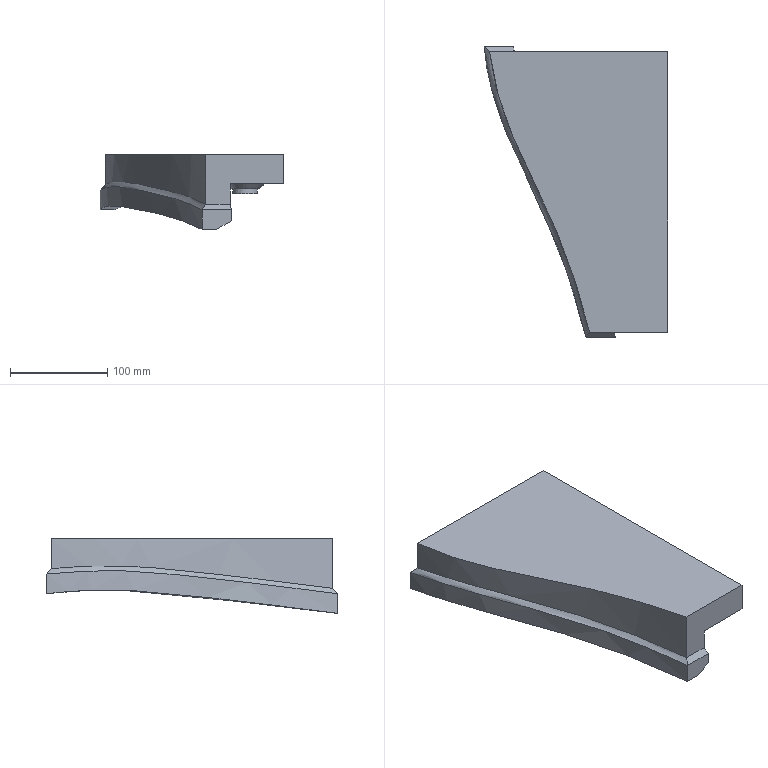Part | NX | features solid 2 | 1 solid | 29 faces | box 188.769 x 298.643 x 76.769 mm | volume 1444145 mm3 | plane 15 | spline 6 | cone 6 | cylinder 2 | commonest cylinder face diameters 25 x2